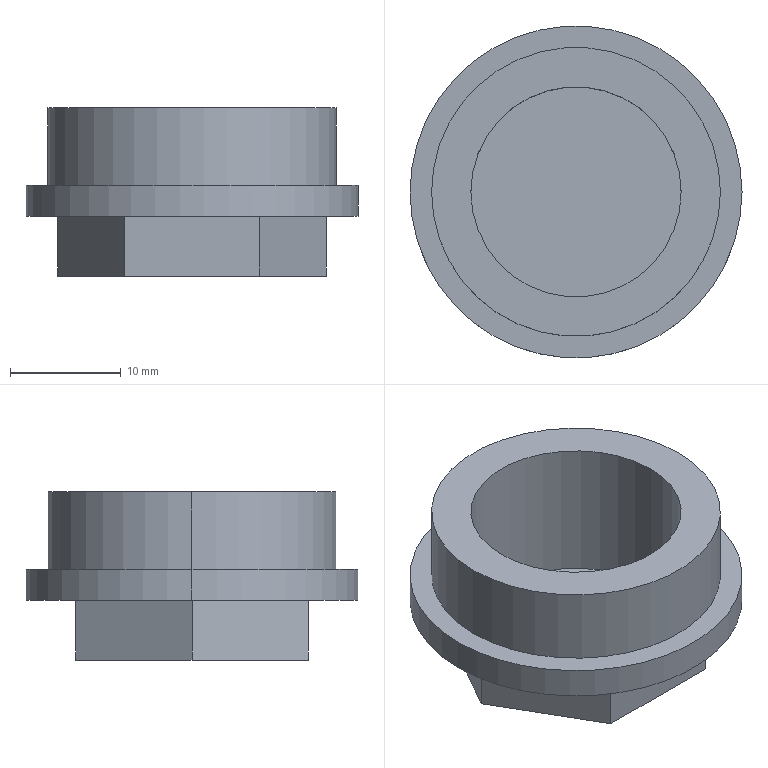Part | SolidWorks | features ICE 3, Extrusion 1 | 1 solid | 17 faces | box 30 x 30 x 15.2 mm | volume 4101 mm3 | plane 11 | cylinder 6 | commonest cylinder face diameters 19 x2 26.1 x2 30 x2
STEP:
#1=CARTESIAN_POINT('',(-9.5,0.,-3.2));
#2=VERTEX_POINT('',#1);
#3=CARTESIAN_POINT('',(9.5,0.,-3.2));
#4=VERTEX_POINT('',#3);
#5=CARTESIAN_POINT('',(0.,0.,-3.2));
#6=DIRECTION('',(0.,0.,1.));
#7=DIRECTION('',(1.,0.,0.));
#8=AXIS2_PLACEMENT_3D('',#5,#6,#7);
#9=CIRCLE('',#8,9.5);
#10=EDGE_CURVE('',#2,#4,#9,.T.);
#11=ORIENTED_EDGE('',*,*,#10,.F.);
#12=CARTESIAN_POINT('',(-9.5,0.,9.8));
#13=VERTEX_POINT('',#12);
#14=CARTESIAN_POINT('',(-9.5,0.,-3.2));
#15=DIRECTION('',(0.,0.,1.));
#16=VECTOR('',#15,1000.);
#17=LINE('',#14,#16);
#18=EDGE_CURVE('',#2,#13,#17,.T.);
#19=ORIENTED_EDGE('',*,*,#18,.T.);
#20=CARTESIAN_POINT('',(9.5,0.,9.8));
#21=VERTEX_POINT('',#20);
#22=CARTESIAN_POINT('',(0.,0.,9.8));
#23=DIRECTION('',(0.,0.,1.));
#24=DIRECTION('',(1.,0.,0.));
#25=AXIS2_PLACEMENT_3D('',#22,#23,#24);
#26=CIRCLE('',#25,9.5);
#27=EDGE_CURVE('',#13,#21,#26,.T.);
#28=ORIENTED_EDGE('',*,*,#27,.T.);
#29=CARTESIAN_POINT('',(9.5,0.,-3.2));
#30=DIRECTION('',(0.,0.,1.));
#31=VECTOR('',#30,1000.);
#32=LINE('',#29,#31);
#33=EDGE_CURVE('',#4,#21,#32,.T.);
#34=ORIENTED_EDGE('',*,*,#33,.F.);
#35=EDGE_LOOP('',(#11,#19,#28,#34));
#36=FACE_OUTER_BOUND('',#35,.T.);
#37=CARTESIAN_POINT('',(0.,0.,-3.2));
#38=DIRECTION('',(0.,0.,1.));
#39=DIRECTION('',(1.,0.,0.));
#40=AXIS2_PLACEMENT_3D('',#37,#38,#39);
#41=CYLINDRICAL_SURFACE('',#40,9.5);
#42=ADVANCED_FACE('',(#36),#41,.F.);
#43=CARTESIAN_POINT('',(13.05,0.,9.8));
#44=VERTEX_POINT('',#43);
#45=CARTESIAN_POINT('',(-13.05,0.,9.8));
#46=VERTEX_POINT('',#45);
#47=CARTESIAN_POINT('',(0.,0.,9.8));
#48=DIRECTION('',(0.,0.,1.));
#49=DIRECTION('',(1.,0.,0.));
#50=AXIS2_PLACEMENT_3D('',#47,#48,#49);
#51=CIRCLE('',#50,13.05);
#52=EDGE_CURVE('',#44,#46,#51,.T.);
#53=ORIENTED_EDGE('',*,*,#52,.F.);
#54=CARTESIAN_POINT('',(13.05,0.,2.8));
#55=VERTEX_POINT('',#54);
#56=CARTESIAN_POINT('',(13.05,0.,9.8));
#57=DIRECTION('',(0.,0.,-1.));
#58=VECTOR('',#57,1000.);
#59=LINE('',#56,#58);
#60=EDGE_CURVE('',#44,#55,#59,.T.);
#61=ORIENTED_EDGE('',*,*,#60,.T.);
#62=CARTESIAN_POINT('',(-13.05,0.,2.8));
#63=VERTEX_POINT('',#62);
#64=CARTESIAN_POINT('',(0.,0.,2.8));
#65=DIRECTION('',(0.,0.,1.));
#66=DIRECTION('',(1.,0.,0.));
#67=AXIS2_PLACEMENT_3D('',#64,#65,#66);
#68=CIRCLE('',#67,13.05);
#69=EDGE_CURVE('',#55,#63,#68,.T.);
#70=ORIENTED_EDGE('',*,*,#69,.T.);
#71=CARTESIAN_POINT('',(-13.05,0.,9.8));
#72=DIRECTION('',(0.,0.,-1.));
#73=VECTOR('',#72,1000.);
#74=LINE('',#71,#73);
#75=EDGE_CURVE('',#46,#63,#74,.T.);
#76=ORIENTED_EDGE('',*,*,#75,.F.);
#77=EDGE_LOOP('',(#53,#61,#70,#76));
#78=FACE_OUTER_BOUND('',#77,.T.);
#79=CARTESIAN_POINT('',(0.,0.,9.8));
#80=DIRECTION('',(0.,0.,-1.));
#81=DIRECTION('',(-1.,0.,0.));
#82=AXIS2_PLACEMENT_3D('',#79,#80,#81);
#83=CYLINDRICAL_SURFACE('',#82,13.05);
#84=ADVANCED_FACE('',(#78),#83,.T.);
#85=CARTESIAN_POINT('',(15.,0.,2.8));
#86=VERTEX_POINT('',#85);
#87=CARTESIAN_POINT('',(-15.,0.,2.8));
#88=VERTEX_POINT('',#87);
#89=CARTESIAN_POINT('',(0.,0.,2.8));
#90=DIRECTION('',(0.,0.,1.));
#91=DIRECTION('',(1.,0.,0.));
#92=AXIS2_PLACEMENT_3D('',#89,#90,#91);
#93=CIRCLE('',#92,15.);
#94=EDGE_CURVE('',#86,#88,#93,.T.);
#95=ORIENTED_EDGE('',*,*,#94,.F.);
#96=CARTESIAN_POINT('',(15.,0.,0.));
#97=VERTEX_POINT('',#96);
#98=CARTESIAN_POINT('',(15.,0.,2.8));
#99=DIRECTION('',(0.,0.,-1.));
#100=VECTOR('',#99,1000.);
#101=LINE('',#98,#100);
#102=EDGE_CURVE('',#86,#97,#101,.T.);
#103=ORIENTED_EDGE('',*,*,#102,.T.);
#104=CARTESIAN_POINT('',(-15.,0.,0.));
#105=VERTEX_POINT('',#104);
#106=CARTESIAN_POINT('',(0.,0.,0.));
#107=DIRECTION('',(0.,0.,1.));
#108=DIRECTION('',(1.,0.,0.));
#109=AXIS2_PLACEMENT_3D('',#106,#107,#108);
#110=CIRCLE('',#109,15.);
#111=EDGE_CURVE('',#97,#105,#110,.T.);
#112=ORIENTED_EDGE('',*,*,#111,.T.);
#113=CARTESIAN_POINT('',(-15.,0.,2.8));
#114=DIRECTION('',(0.,0.,-1.));
#115=VECTOR('',#114,1000.);
#116=LINE('',#113,#115);
#117=EDGE_CURVE('',#88,#105,#116,.T.);
#118=ORIENTED_EDGE('',*,*,#117,.F.);
#119=EDGE_LOOP('',(#95,#103,#112,#118));
#120=FACE_OUTER_BOUND('',#119,.T.);
#121=CARTESIAN_POINT('',(0.,0.,2.8));
#122=DIRECTION('',(0.,0.,-1.));
#123=DIRECTION('',(-1.,0.,0.));
#124=AXIS2_PLACEMENT_3D('',#121,#122,#123);
#125=CYLINDRICAL_SURFACE('',#124,15.);
#126=ADVANCED_FACE('',(#120),#125,.T.);
#127=CARTESIAN_POINT('',(0.,0.,0.));
#128=DIRECTION('',(0.,0.,1.));
#129=DIRECTION('',(1.,0.,0.));
#130=AXIS2_PLACEMENT_3D('',#127,#128,#129);
#131=CIRCLE('',#130,15.);
#132=EDGE_CURVE('',#105,#97,#131,.T.);
#133=ORIENTED_EDGE('',*,*,#132,.F.);
#134=ORIENTED_EDGE('',*,*,#111,.F.);
#135=EDGE_LOOP('',(#133,#134));
#136=FACE_OUTER_BOUND('',#135,.T.);
#137=CARTESIAN_POINT('',(6.062,-10.5,0.));
#138=VERTEX_POINT('',#137);
#139=CARTESIAN_POINT('',(-6.062,-10.5,0.));
#140=VERTEX_POINT('',#139);
#141=CARTESIAN_POINT('',(6.062,-10.5,0.));
#142=DIRECTION('',(-1.,0.,0.));
#143=VECTOR('',#142,1000.);
#144=LINE('',#141,#143);
#145=EDGE_CURVE('',#138,#140,#144,.T.);
#146=ORIENTED_EDGE('',*,*,#145,.F.);
#147=CARTESIAN_POINT('',(12.124,0.,0.));
#148=VERTEX_POINT('',#147);
#149=CARTESIAN_POINT('',(12.124,0.,0.));
#150=DIRECTION('',(-0.5,-0.866,0.));
#151=VECTOR('',#150,1000.);
#152=LINE('',#149,#151);
#153=EDGE_CURVE('',#148,#138,#152,.T.);
#154=ORIENTED_EDGE('',*,*,#153,.F.);
#155=CARTESIAN_POINT('',(6.062,10.5,0.));
#156=VERTEX_POINT('',#155);
#157=CARTESIAN_POINT('',(6.062,10.5,0.));
#158=DIRECTION('',(0.5,-0.866,0.));
#159=VECTOR('',#158,1000.);
#160=LINE('',#157,#159);
#161=EDGE_CURVE('',#156,#148,#160,.T.);
#162=ORIENTED_EDGE('',*,*,#161,.F.);
#163=CARTESIAN_POINT('',(-6.062,10.5,0.));
#164=VERTEX_POINT('',#163);
#165=CARTESIAN_POINT('',(-6.062,10.5,0.));
#166=DIRECTION('',(1.,0.,0.));
#167=VECTOR('',#166,1000.);
#168=LINE('',#165,#167);
#169=EDGE_CURVE('',#164,#156,#168,.T.);
#170=ORIENTED_EDGE('',*,*,#169,.F.);
#171=CARTESIAN_POINT('',(-12.124,0.,0.));
#172=VERTEX_POINT('',#171);
#173=CARTESIAN_POINT('',(-12.124,0.,0.));
#174=DIRECTION('',(0.5,0.866,0.));
#175=VECTOR('',#174,1000.);
#176=LINE('',#173,#175);
#177=EDGE_CURVE('',#172,#164,#176,.T.);
#178=ORIENTED_EDGE('',*,*,#177,.F.);
#179=CARTESIAN_POINT('',(-6.062,-10.5,0.));
#180=DIRECTION('',(-0.5,0.866,0.));
#181=VECTOR('',#180,1000.);
#182=LINE('',#179,#181);
#183=EDGE_CURVE('',#140,#172,#182,.T.);
#184=ORIENTED_EDGE('',*,*,#183,.F.);
#185=EDGE_LOOP('',(#146,#154,#162,#170,#178,#184));
#186=FACE_BOUND('',#185,.T.);
#187=CARTESIAN_POINT('',(0.,0.,0.));
#188=DIRECTION('',(0.,0.,1.));
#189=DIRECTION('',(1.,0.,0.));
#190=AXIS2_PLACEMENT_3D('',#187,#188,#189);
#191=PLANE('',#190);
#192=ADVANCED_FACE('',(#136,#186),#191,.F.);
#193=ORIENTED_EDGE('',*,*,#102,.F.);
#194=CARTESIAN_POINT('',(0.,0.,2.8));
#195=DIRECTION('',(0.,0.,1.));
#196=DIRECTION('',(1.,0.,0.));
#197=AXIS2_PLACEMENT_3D('',#194,#195,#196);
#198=CIRCLE('',#197,15.);
#199=EDGE_CURVE('',#88,#86,#198,.T.);
#200=ORIENTED_EDGE('',*,*,#199,.F.);
#201=ORIENTED_EDGE('',*,*,#117,.T.);
#202=ORIENTED_EDGE('',*,*,#132,.T.);
#203=EDGE_LOOP('',(#193,#200,#201,#202));
#204=FACE_OUTER_BOUND('',#203,.T.);
#205=CARTESIAN_POINT('',(0.,0.,2.8));
#206=DIRECTION('',(0.,0.,-1.));
#207=DIRECTION('',(-1.,0.,0.));
#208=AXIS2_PLACEMENT_3D('',#205,#206,#207);
#209=CYLINDRICAL_SURFACE('',#208,15.);
#210=ADVANCED_FACE('',(#204),#209,.T.);
#211=CARTESIAN_POINT('',(0.,0.,2.8));
#212=DIRECTION('',(0.,0.,1.));
#213=DIRECTION('',(1.,0.,0.));
#214=AXIS2_PLACEMENT_3D('',#211,#212,#213);
#215=CIRCLE('',#214,13.05);
#216=EDGE_CURVE('',#63,#55,#215,.T.);
#217=ORIENTED_EDGE('',*,*,#216,.F.);
#218=ORIENTED_EDGE('',*,*,#69,.F.);
#219=EDGE_LOOP('',(#217,#218));
#220=FACE_BOUND('',#219,.T.);
#221=ORIENTED_EDGE('',*,*,#199,.T.);
#222=ORIENTED_EDGE('',*,*,#94,.T.);
#223=EDGE_LOOP('',(#221,#222));
#224=FACE_OUTER_BOUND('',#223,.T.);
#225=CARTESIAN_POINT('',(0.,0.,2.8));
#226=DIRECTION('',(0.,0.,1.));
#227=DIRECTION('',(1.,0.,0.));
#228=AXIS2_PLACEMENT_3D('',#225,#226,#227);
#229=PLANE('',#228);
#230=ADVANCED_FACE('',(#220,#224),#229,.T.);
#231=ORIENTED_EDGE('',*,*,#145,.T.);
#232=CARTESIAN_POINT('',(-6.062,-10.5,-5.4));
#233=VERTEX_POINT('',#232);
#234=CARTESIAN_POINT('',(-6.062,-10.5,-5.4));
#235=DIRECTION('',(0.,0.,1.));
#236=VECTOR('',#235,1000.);
#237=LINE('',#234,#236);
#238=EDGE_CURVE('',#233,#140,#237,.T.);
#239=ORIENTED_EDGE('',*,*,#238,.F.);
#240=CARTESIAN_POINT('',(6.062,-10.5,-5.4));
#241=VERTEX_POINT('',#240);
#242=CARTESIAN_POINT('',(6.062,-10.5,-5.4));
#243=DIRECTION('',(-1.,0.,0.));
#244=VECTOR('',#243,1000.);
#245=LINE('',#242,#244);
#246=EDGE_CURVE('',#241,#233,#245,.T.);
#247=ORIENTED_EDGE('',*,*,#246,.F.);
#248=CARTESIAN_POINT('',(6.062,-10.5,-5.4));
#249=DIRECTION('',(0.,0.,1.));
#250=VECTOR('',#249,1000.);
#251=LINE('',#248,#250);
#252=EDGE_CURVE('',#241,#138,#251,.T.);
#253=ORIENTED_EDGE('',*,*,#252,.T.);
#254=EDGE_LOOP('',(#231,#239,#247,#253));
#255=FACE_OUTER_BOUND('',#254,.T.);
#256=CARTESIAN_POINT('',(6.062,-10.5,-5.4));
#257=DIRECTION('',(0.,1.,0.));
#258=DIRECTION('',(0.,0.,1.));
#259=AXIS2_PLACEMENT_3D('',#256,#257,#258);
#260=PLANE('',#259);
#261=ADVANCED_FACE('',(#255),#260,.F.);
#262=ORIENTED_EDGE('',*,*,#183,.T.);
#263=CARTESIAN_POINT('',(-12.124,0.,-5.4));
#264=VERTEX_POINT('',#263);
#265=CARTESIAN_POINT('',(-12.124,0.,-5.4));
#266=DIRECTION('',(0.,0.,1.));
#267=VECTOR('',#266,1000.);
#268=LINE('',#265,#267);
#269=EDGE_CURVE('',#264,#172,#268,.T.);
#270=ORIENTED_EDGE('',*,*,#269,.F.);
#271=CARTESIAN_POINT('',(-6.062,-10.5,-5.4));
#272=DIRECTION('',(-0.5,0.866,0.));
#273=VECTOR('',#272,1000.);
#274=LINE('',#271,#273);
#275=EDGE_CURVE('',#233,#264,#274,.T.);
#276=ORIENTED_EDGE('',*,*,#275,.F.);
#277=ORIENTED_EDGE('',*,*,#238,.T.);
#278=EDGE_LOOP('',(#262,#270,#276,#277));
#279=FACE_OUTER_BOUND('',#278,.T.);
#280=CARTESIAN_POINT('',(-6.062,-10.5,-5.4));
#281=DIRECTION('',(0.866,0.5,0.));
#282=DIRECTION('',(-0.5,0.866,0.));
#283=AXIS2_PLACEMENT_3D('',#280,#281,#282);
#284=PLANE('',#283);
#285=ADVANCED_FACE('',(#279),#284,.F.);
#286=ORIENTED_EDGE('',*,*,#177,.T.);
#287=CARTESIAN_POINT('',(-6.062,10.5,-5.4));
#288=VERTEX_POINT('',#287);
#289=CARTESIAN_POINT('',(-6.062,10.5,-5.4));
#290=DIRECTION('',(0.,0.,1.));
#291=VECTOR('',#290,1000.);
#292=LINE('',#289,#291);
#293=EDGE_CURVE('',#288,#164,#292,.T.);
#294=ORIENTED_EDGE('',*,*,#293,.F.);
#295=CARTESIAN_POINT('',(-12.124,0.,-5.4));
#296=DIRECTION('',(0.5,0.866,0.));
#297=VECTOR('',#296,1000.);
#298=LINE('',#295,#297);
#299=EDGE_CURVE('',#264,#288,#298,.T.);
#300=ORIENTED_EDGE('',*,*,#299,.F.);
#301=ORIENTED_EDGE('',*,*,#269,.T.);
#302=EDGE_LOOP('',(#286,#294,#300,#301));
#303=FACE_OUTER_BOUND('',#302,.T.);
#304=CARTESIAN_POINT('',(-12.124,0.,-5.4));
#305=DIRECTION('',(0.866,-0.5,0.));
#306=DIRECTION('',(0.5,0.866,0.));
#307=AXIS2_PLACEMENT_3D('',#304,#305,#306);
#308=PLANE('',#307);
#309=ADVANCED_FACE('',(#303),#308,.F.);
#310=ORIENTED_EDGE('',*,*,#169,.T.);
#311=CARTESIAN_POINT('',(6.062,10.5,-5.4));
#312=VERTEX_POINT('',#311);
#313=CARTESIAN_POINT('',(6.062,10.5,-5.4));
#314=DIRECTION('',(0.,0.,1.));
#315=VECTOR('',#314,1000.);
#316=LINE('',#313,#315);
#317=EDGE_CURVE('',#312,#156,#316,.T.);
#318=ORIENTED_EDGE('',*,*,#317,.F.);
#319=CARTESIAN_POINT('',(-6.062,10.5,-5.4));
#320=DIRECTION('',(1.,0.,0.));
#321=VECTOR('',#320,1000.);
#322=LINE('',#319,#321);
#323=EDGE_CURVE('',#288,#312,#322,.T.);
#324=ORIENTED_EDGE('',*,*,#323,.F.);
#325=ORIENTED_EDGE('',*,*,#293,.T.);
#326=EDGE_LOOP('',(#310,#318,#324,#325));
#327=FACE_OUTER_BOUND('',#326,.T.);
#328=CARTESIAN_POINT('',(-6.062,10.5,-5.4));
#329=DIRECTION('',(0.,-1.,0.));
#330=DIRECTION('',(0.,0.,-1.));
#331=AXIS2_PLACEMENT_3D('',#328,#329,#330);
#332=PLANE('',#331);
#333=ADVANCED_FACE('',(#327),#332,.F.);
#334=ORIENTED_EDGE('',*,*,#161,.T.);
#335=CARTESIAN_POINT('',(12.124,0.,-5.4));
#336=VERTEX_POINT('',#335);
#337=CARTESIAN_POINT('',(12.124,0.,-5.4));
#338=DIRECTION('',(0.,0.,1.));
#339=VECTOR('',#338,1000.);
#340=LINE('',#337,#339);
#341=EDGE_CURVE('',#336,#148,#340,.T.);
#342=ORIENTED_EDGE('',*,*,#341,.F.);
#343=CARTESIAN_POINT('',(6.062,10.5,-5.4));
#344=DIRECTION('',(0.5,-0.866,0.));
#345=VECTOR('',#344,1000.);
#346=LINE('',#343,#345);
#347=EDGE_CURVE('',#312,#336,#346,.T.);
#348=ORIENTED_EDGE('',*,*,#347,.F.);
#349=ORIENTED_EDGE('',*,*,#317,.T.);
#350=EDGE_LOOP('',(#334,#342,#348,#349));
#351=FACE_OUTER_BOUND('',#350,.T.);
#352=CARTESIAN_POINT('',(6.062,10.5,-5.4));
#353=DIRECTION('',(-0.866,-0.5,0.));
#354=DIRECTION('',(0.5,-0.866,0.));
#355=AXIS2_PLACEMENT_3D('',#352,#353,#354);
#356=PLANE('',#355);
#357=ADVANCED_FACE('',(#351),#356,.F.);
#358=ORIENTED_EDGE('',*,*,#153,.T.);
#359=ORIENTED_EDGE('',*,*,#252,.F.);
#360=CARTESIAN_POINT('',(12.124,0.,-5.4));
#361=DIRECTION('',(-0.5,-0.866,0.));
#362=VECTOR('',#361,1000.);
#363=LINE('',#360,#362);
#364=EDGE_CURVE('',#336,#241,#363,.T.);
#365=ORIENTED_EDGE('',*,*,#364,.F.);
#366=ORIENTED_EDGE('',*,*,#341,.T.);
#367=EDGE_LOOP('',(#358,#359,#365,#366));
#368=FACE_OUTER_BOUND('',#367,.T.);
#369=CARTESIAN_POINT('',(12.124,0.,-5.4));
#370=DIRECTION('',(-0.866,0.5,0.));
#371=DIRECTION('',(-0.5,-0.866,0.));
#372=AXIS2_PLACEMENT_3D('',#369,#370,#371);
#373=PLANE('',#372);
#374=ADVANCED_FACE('',(#368),#373,.F.);
#375=ORIENTED_EDGE('',*,*,#246,.T.);
#376=ORIENTED_EDGE('',*,*,#275,.T.);
#377=ORIENTED_EDGE('',*,*,#299,.T.);
#378=ORIENTED_EDGE('',*,*,#323,.T.);
#379=ORIENTED_EDGE('',*,*,#347,.T.);
#380=ORIENTED_EDGE('',*,*,#364,.T.);
#381=EDGE_LOOP('',(#375,#376,#377,#378,#379,#380));
#382=FACE_OUTER_BOUND('',#381,.T.);
#383=CARTESIAN_POINT('',(0.,0.,-5.4));
#384=DIRECTION('',(0.,0.,-1.));
#385=DIRECTION('',(-1.,0.,0.));
#386=AXIS2_PLACEMENT_3D('',#383,#384,#385);
#387=PLANE('',#386);
#388=ADVANCED_FACE('',(#382),#387,.T.);
#389=ORIENTED_EDGE('',*,*,#60,.F.);
#390=CARTESIAN_POINT('',(0.,0.,9.8));
#391=DIRECTION('',(0.,0.,1.));
#392=DIRECTION('',(1.,0.,0.));
#393=AXIS2_PLACEMENT_3D('',#390,#391,#392);
#394=CIRCLE('',#393,13.05);
#395=EDGE_CURVE('',#46,#44,#394,.T.);
#396=ORIENTED_EDGE('',*,*,#395,.F.);
#397=ORIENTED_EDGE('',*,*,#75,.T.);
#398=ORIENTED_EDGE('',*,*,#216,.T.);
#399=EDGE_LOOP('',(#389,#396,#397,#398));
#400=FACE_OUTER_BOUND('',#399,.T.);
#401=CARTESIAN_POINT('',(0.,0.,9.8));
#402=DIRECTION('',(0.,0.,-1.));
#403=DIRECTION('',(-1.,0.,0.));
#404=AXIS2_PLACEMENT_3D('',#401,#402,#403);
#405=CYLINDRICAL_SURFACE('',#404,13.05);
#406=ADVANCED_FACE('',(#400),#405,.T.);
#407=CARTESIAN_POINT('',(0.,0.,9.8));
#408=DIRECTION('',(0.,0.,1.));
#409=DIRECTION('',(1.,0.,0.));
#410=AXIS2_PLACEMENT_3D('',#407,#408,#409);
#411=CIRCLE('',#410,9.5);
#412=EDGE_CURVE('',#21,#13,#411,.T.);
#413=ORIENTED_EDGE('',*,*,#412,.F.);
#414=ORIENTED_EDGE('',*,*,#27,.F.);
#415=EDGE_LOOP('',(#413,#414));
#416=FACE_BOUND('',#415,.T.);
#417=ORIENTED_EDGE('',*,*,#395,.T.);
#418=ORIENTED_EDGE('',*,*,#52,.T.);
#419=EDGE_LOOP('',(#417,#418));
#420=FACE_OUTER_BOUND('',#419,.T.);
#421=CARTESIAN_POINT('',(0.,0.,9.8));
#422=DIRECTION('',(0.,0.,1.));
#423=DIRECTION('',(1.,0.,0.));
#424=AXIS2_PLACEMENT_3D('',#421,#422,#423);
#425=PLANE('',#424);
#426=ADVANCED_FACE('',(#416,#420),#425,.T.);
#427=ORIENTED_EDGE('',*,*,#18,.F.);
#428=CARTESIAN_POINT('',(0.,0.,-3.2));
#429=DIRECTION('',(0.,0.,1.));
#430=DIRECTION('',(1.,0.,0.));
#431=AXIS2_PLACEMENT_3D('',#428,#429,#430);
#432=CIRCLE('',#431,9.5);
#433=EDGE_CURVE('',#4,#2,#432,.T.);
#434=ORIENTED_EDGE('',*,*,#433,.F.);
#435=ORIENTED_EDGE('',*,*,#33,.T.);
#436=ORIENTED_EDGE('',*,*,#412,.T.);
#437=EDGE_LOOP('',(#427,#434,#435,#436));
#438=FACE_OUTER_BOUND('',#437,.T.);
#439=CARTESIAN_POINT('',(0.,0.,-3.2));
#440=DIRECTION('',(0.,0.,1.));
#441=DIRECTION('',(1.,0.,0.));
#442=AXIS2_PLACEMENT_3D('',#439,#440,#441);
#443=CYLINDRICAL_SURFACE('',#442,9.5);
#444=ADVANCED_FACE('',(#438),#443,.F.);
#445=ORIENTED_EDGE('',*,*,#433,.T.);
#446=ORIENTED_EDGE('',*,*,#10,.T.);
#447=EDGE_LOOP('',(#445,#446));
#448=FACE_OUTER_BOUND('',#447,.T.);
#449=CARTESIAN_POINT('',(0.,0.,-3.2));
#450=DIRECTION('',(0.,0.,1.));
#451=DIRECTION('',(1.,0.,0.));
#452=AXIS2_PLACEMENT_3D('',#449,#450,#451);
#453=PLANE('',#452);
#454=ADVANCED_FACE('',(#448),#453,.T.);
#455=CLOSED_SHELL('',(#42,#84,#126,#192,#210,#230,#261,#285,#309,#333,#357,#374,#388,#406,#426,#444,#454));
#456=MANIFOLD_SOLID_BREP('',#455);
#457=CARTESIAN_POINT('',(0.,0.,0.));
#458=DIRECTION('',(0.,0.,1.));
#459=DIRECTION('',(1.,0.,0.));
#460=AXIS2_PLACEMENT_3D('',#457,#458,#459);
#461=(LENGTH_UNIT()NAMED_UNIT(*)SI_UNIT(.MILLI.,.METRE.));
#462=UNCERTAINTY_MEASURE_WITH_UNIT(LENGTH_MEASURE(0.00001),#461,'','');
#463=(NAMED_UNIT(*)PLANE_ANGLE_UNIT()SI_UNIT($,.RADIAN.));
#464=(NAMED_UNIT(*)SI_UNIT($,.STERADIAN.)SOLID_ANGLE_UNIT());
#465=(GEOMETRIC_REPRESENTATION_CONTEXT(3)GLOBAL_UNCERTAINTY_ASSIGNED_CONTEXT((#462))GLOBAL_UNIT_ASSIGNED_CONTEXT((#461,#463,#464))REPRESENTATION_CONTEXT('',''));
#466=ADVANCED_BREP_SHAPE_REPRESENTATION('',(#456,#460),#465);